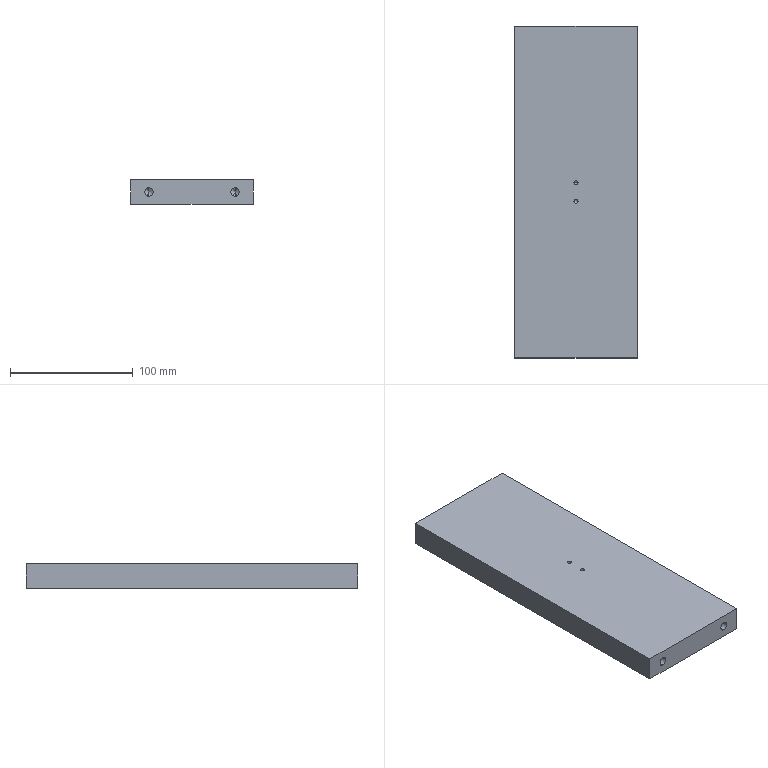Part | SolidWorks | features HoleWzd 3, 3DProfileFeature 1, Extrusion 1 | 1 solid | 42 faces | box 100 x 270 x 20 mm | volume 536586 mm3 | cylinder 18 | cone 18 | plane 6 | commonest cylinder face diameters 3.3 x10 6.8 x8
STEP:
#1=CARTESIAN_POINT('',(61.65,-55.,10.1));
#2=VERTEX_POINT('',#1);
#3=CARTESIAN_POINT('',(58.35,-55.,10.1));
#4=VERTEX_POINT('',#3);
#5=CARTESIAN_POINT('',(60.,-55.,10.1));
#6=DIRECTION('',(0.,0.,-1.));
#7=DIRECTION('',(-1.,0.,0.));
#8=AXIS2_PLACEMENT_3D('',#5,#6,#7);
#9=CIRCLE('',#8,1.65);
#10=EDGE_CURVE('',#2,#4,#9,.T.);
#11=ORIENTED_EDGE('',*,*,#10,.F.);
#12=CARTESIAN_POINT('',(61.65,-55.,0.));
#13=VERTEX_POINT('',#12);
#14=CARTESIAN_POINT('',(61.65,-55.,0.));
#15=DIRECTION('',(0.,0.,-1.));
#16=VECTOR('',#15,1000.);
#17=LINE('',#14,#16);
#18=EDGE_CURVE('',#2,#13,#17,.T.);
#19=ORIENTED_EDGE('',*,*,#18,.T.);
#20=CARTESIAN_POINT('',(58.35,-55.,0.));
#21=VERTEX_POINT('',#20);
#22=CARTESIAN_POINT('',(60.,-55.,0.));
#23=DIRECTION('',(0.,0.,-1.));
#24=DIRECTION('',(-1.,0.,0.));
#25=AXIS2_PLACEMENT_3D('',#22,#23,#24);
#26=CIRCLE('',#25,1.65);
#27=EDGE_CURVE('',#13,#21,#26,.T.);
#28=ORIENTED_EDGE('',*,*,#27,.T.);
#29=CARTESIAN_POINT('',(58.35,-55.,0.));
#30=DIRECTION('',(0.,0.,-1.));
#31=VECTOR('',#30,1000.);
#32=LINE('',#29,#31);
#33=EDGE_CURVE('',#4,#21,#32,.T.);
#34=ORIENTED_EDGE('',*,*,#33,.F.);
#35=EDGE_LOOP('',(#11,#19,#28,#34));
#36=FACE_OUTER_BOUND('',#35,.T.);
#37=CARTESIAN_POINT('',(60.,-55.,0.));
#38=DIRECTION('',(0.,0.,-1.));
#39=DIRECTION('',(-1.,0.,0.));
#40=AXIS2_PLACEMENT_3D('',#37,#38,#39);
#41=CYLINDRICAL_SURFACE('',#40,1.65);
#42=ADVANCED_FACE('',(#36),#41,.F.);
#43=CARTESIAN_POINT('',(60.,-55.,11.091));
#44=VERTEX_POINT('',#43);
#45=CARTESIAN_POINT('',(58.35,-55.,10.1));
#46=DIRECTION('',(-0.8572,0.,-0.515));
#47=VECTOR('',#46,1000.);
#48=LINE('',#45,#47);
#49=EDGE_CURVE('',#44,#4,#48,.T.);
#50=ORIENTED_EDGE('',*,*,#49,.F.);
#51=CARTESIAN_POINT('',(61.65,-55.,10.1));
#52=DIRECTION('',(0.8572,0.,-0.515));
#53=VECTOR('',#52,1000.);
#54=LINE('',#51,#53);
#55=EDGE_CURVE('',#44,#2,#54,.T.);
#56=ORIENTED_EDGE('',*,*,#55,.T.);
#57=ORIENTED_EDGE('',*,*,#10,.T.);
#58=EDGE_LOOP('',(#50,#56,#57));
#59=FACE_OUTER_BOUND('',#58,.T.);
#60=CARTESIAN_POINT('',(60.,-55.,10.1));
#61=DIRECTION('',(0.,0.,-1.));
#62=DIRECTION('',(-1.,0.,0.));
#63=AXIS2_PLACEMENT_3D('',#60,#61,#62);
#64=CONICAL_SURFACE('',#63,1.65,1.03);
#65=ADVANCED_FACE('',(#59),#64,.F.);
#66=CARTESIAN_POINT('',(61.65,-115.,10.1));
#67=VERTEX_POINT('',#66);
#68=CARTESIAN_POINT('',(58.35,-115.,10.1));
#69=VERTEX_POINT('',#68);
#70=CARTESIAN_POINT('',(60.,-115.,10.1));
#71=DIRECTION('',(0.,0.,-1.));
#72=DIRECTION('',(-1.,0.,0.));
#73=AXIS2_PLACEMENT_3D('',#70,#71,#72);
#74=CIRCLE('',#73,1.65);
#75=EDGE_CURVE('',#67,#69,#74,.T.);
#76=ORIENTED_EDGE('',*,*,#75,.F.);
#77=CARTESIAN_POINT('',(61.65,-115.,0.));
#78=VERTEX_POINT('',#77);
#79=CARTESIAN_POINT('',(61.65,-115.,0.));
#80=DIRECTION('',(0.,0.,-1.));
#81=VECTOR('',#80,1000.);
#82=LINE('',#79,#81);
#83=EDGE_CURVE('',#67,#78,#82,.T.);
#84=ORIENTED_EDGE('',*,*,#83,.T.);
#85=CARTESIAN_POINT('',(58.35,-115.,0.));
#86=VERTEX_POINT('',#85);
#87=CARTESIAN_POINT('',(60.,-115.,0.));
#88=DIRECTION('',(0.,0.,-1.));
#89=DIRECTION('',(-1.,0.,0.));
#90=AXIS2_PLACEMENT_3D('',#87,#88,#89);
#91=CIRCLE('',#90,1.65);
#92=EDGE_CURVE('',#78,#86,#91,.T.);
#93=ORIENTED_EDGE('',*,*,#92,.T.);
#94=CARTESIAN_POINT('',(58.35,-115.,0.));
#95=DIRECTION('',(0.,0.,-1.));
#96=VECTOR('',#95,1000.);
#97=LINE('',#94,#96);
#98=EDGE_CURVE('',#69,#86,#97,.T.);
#99=ORIENTED_EDGE('',*,*,#98,.F.);
#100=EDGE_LOOP('',(#76,#84,#93,#99));
#101=FACE_OUTER_BOUND('',#100,.T.);
#102=CARTESIAN_POINT('',(60.,-115.,0.));
#103=DIRECTION('',(0.,0.,-1.));
#104=DIRECTION('',(-1.,0.,0.));
#105=AXIS2_PLACEMENT_3D('',#102,#103,#104);
#106=CYLINDRICAL_SURFACE('',#105,1.65);
#107=ADVANCED_FACE('',(#101),#106,.F.);
#108=CARTESIAN_POINT('',(60.,-115.,11.091));
#109=VERTEX_POINT('',#108);
#110=CARTESIAN_POINT('',(58.35,-115.,10.1));
#111=DIRECTION('',(-0.8572,0.,-0.515));
#112=VECTOR('',#111,1000.);
#113=LINE('',#110,#112);
#114=EDGE_CURVE('',#109,#69,#113,.T.);
#115=ORIENTED_EDGE('',*,*,#114,.F.);
#116=CARTESIAN_POINT('',(61.65,-115.,10.1));
#117=DIRECTION('',(0.8572,0.,-0.515));
#118=VECTOR('',#117,1000.);
#119=LINE('',#116,#118);
#120=EDGE_CURVE('',#109,#67,#119,.T.);
#121=ORIENTED_EDGE('',*,*,#120,.T.);
#122=ORIENTED_EDGE('',*,*,#75,.T.);
#123=EDGE_LOOP('',(#115,#121,#122));
#124=FACE_OUTER_BOUND('',#123,.T.);
#125=CARTESIAN_POINT('',(60.,-115.,10.1));
#126=DIRECTION('',(0.,0.,-1.));
#127=DIRECTION('',(-1.,0.,0.));
#128=AXIS2_PLACEMENT_3D('',#125,#126,#127);
#129=CONICAL_SURFACE('',#128,1.65,1.03);
#130=ADVANCED_FACE('',(#124),#129,.F.);
#131=CARTESIAN_POINT('',(61.65,-175.,10.1));
#132=VERTEX_POINT('',#131);
#133=CARTESIAN_POINT('',(58.35,-175.,10.1));
#134=VERTEX_POINT('',#133);
#135=CARTESIAN_POINT('',(60.,-175.,10.1));
#136=DIRECTION('',(0.,0.,-1.));
#137=DIRECTION('',(-1.,0.,0.));
#138=AXIS2_PLACEMENT_3D('',#135,#136,#137);
#139=CIRCLE('',#138,1.65);
#140=EDGE_CURVE('',#132,#134,#139,.T.);
#141=ORIENTED_EDGE('',*,*,#140,.F.);
#142=CARTESIAN_POINT('',(61.65,-175.,0.));
#143=VERTEX_POINT('',#142);
#144=CARTESIAN_POINT('',(61.65,-175.,0.));
#145=DIRECTION('',(0.,0.,-1.));
#146=VECTOR('',#145,1000.);
#147=LINE('',#144,#146);
#148=EDGE_CURVE('',#132,#143,#147,.T.);
#149=ORIENTED_EDGE('',*,*,#148,.T.);
#150=CARTESIAN_POINT('',(58.35,-175.,0.));
#151=VERTEX_POINT('',#150);
#152=CARTESIAN_POINT('',(60.,-175.,0.));
#153=DIRECTION('',(0.,0.,-1.));
#154=DIRECTION('',(-1.,0.,0.));
#155=AXIS2_PLACEMENT_3D('',#152,#153,#154);
#156=CIRCLE('',#155,1.65);
#157=EDGE_CURVE('',#143,#151,#156,.T.);
#158=ORIENTED_EDGE('',*,*,#157,.T.);
#159=CARTESIAN_POINT('',(58.35,-175.,0.));
#160=DIRECTION('',(0.,0.,-1.));
#161=VECTOR('',#160,1000.);
#162=LINE('',#159,#161);
#163=EDGE_CURVE('',#134,#151,#162,.T.);
#164=ORIENTED_EDGE('',*,*,#163,.F.);
#165=EDGE_LOOP('',(#141,#149,#158,#164));
#166=FACE_OUTER_BOUND('',#165,.T.);
#167=CARTESIAN_POINT('',(60.,-175.,0.));
#168=DIRECTION('',(0.,0.,-1.));
#169=DIRECTION('',(-1.,0.,0.));
#170=AXIS2_PLACEMENT_3D('',#167,#168,#169);
#171=CYLINDRICAL_SURFACE('',#170,1.65);
#172=ADVANCED_FACE('',(#166),#171,.F.);
#173=CARTESIAN_POINT('',(60.,-175.,11.091));
#174=VERTEX_POINT('',#173);
#175=CARTESIAN_POINT('',(58.35,-175.,10.1));
#176=DIRECTION('',(-0.8572,0.,-0.515));
#177=VECTOR('',#176,1000.);
#178=LINE('',#175,#177);
#179=EDGE_CURVE('',#174,#134,#178,.T.);
#180=ORIENTED_EDGE('',*,*,#179,.F.);
#181=CARTESIAN_POINT('',(61.65,-175.,10.1));
#182=DIRECTION('',(0.8572,0.,-0.515));
#183=VECTOR('',#182,1000.);
#184=LINE('',#181,#183);
#185=EDGE_CURVE('',#174,#132,#184,.T.);
#186=ORIENTED_EDGE('',*,*,#185,.T.);
#187=ORIENTED_EDGE('',*,*,#140,.T.);
#188=EDGE_LOOP('',(#180,#186,#187));
#189=FACE_OUTER_BOUND('',#188,.T.);
#190=CARTESIAN_POINT('',(60.,-175.,10.1));
#191=DIRECTION('',(0.,0.,-1.));
#192=DIRECTION('',(-1.,0.,0.));
#193=AXIS2_PLACEMENT_3D('',#190,#191,#192);
#194=CONICAL_SURFACE('',#193,1.65,1.03);
#195=ADVANCED_FACE('',(#189),#194,.F.);
#196=CARTESIAN_POINT('',(48.35,-127.5,9.9));
#197=VERTEX_POINT('',#196);
#198=CARTESIAN_POINT('',(51.65,-127.5,9.9));
#199=VERTEX_POINT('',#198);
#200=CARTESIAN_POINT('',(50.,-127.5,9.9));
#201=DIRECTION('',(0.,0.,1.));
#202=DIRECTION('',(1.,0.,0.));
#203=AXIS2_PLACEMENT_3D('',#200,#201,#202);
#204=CIRCLE('',#203,1.65);
#205=EDGE_CURVE('',#197,#199,#204,.T.);
#206=ORIENTED_EDGE('',*,*,#205,.F.);
#207=CARTESIAN_POINT('',(48.35,-127.5,20.));
#208=VERTEX_POINT('',#207);
#209=CARTESIAN_POINT('',(48.35,-127.5,20.));
#210=DIRECTION('',(0.,0.,1.));
#211=VECTOR('',#210,1000.);
#212=LINE('',#209,#211);
#213=EDGE_CURVE('',#197,#208,#212,.T.);
#214=ORIENTED_EDGE('',*,*,#213,.T.);
#215=CARTESIAN_POINT('',(51.65,-127.5,20.));
#216=VERTEX_POINT('',#215);
#217=CARTESIAN_POINT('',(50.,-127.5,20.));
#218=DIRECTION('',(0.,0.,1.));
#219=DIRECTION('',(1.,0.,0.));
#220=AXIS2_PLACEMENT_3D('',#217,#218,#219);
#221=CIRCLE('',#220,1.65);
#222=EDGE_CURVE('',#208,#216,#221,.T.);
#223=ORIENTED_EDGE('',*,*,#222,.T.);
#224=CARTESIAN_POINT('',(51.65,-127.5,20.));
#225=DIRECTION('',(0.,0.,1.));
#226=VECTOR('',#225,1000.);
#227=LINE('',#224,#226);
#228=EDGE_CURVE('',#199,#216,#227,.T.);
#229=ORIENTED_EDGE('',*,*,#228,.F.);
#230=EDGE_LOOP('',(#206,#214,#223,#229));
#231=FACE_OUTER_BOUND('',#230,.T.);
#232=CARTESIAN_POINT('',(50.,-127.5,20.));
#233=DIRECTION('',(0.,0.,1.));
#234=DIRECTION('',(1.,0.,0.));
#235=AXIS2_PLACEMENT_3D('',#232,#233,#234);
#236=CYLINDRICAL_SURFACE('',#235,1.65);
#237=ADVANCED_FACE('',(#231),#236,.F.);
#238=CARTESIAN_POINT('',(50.,-127.5,8.909));
#239=VERTEX_POINT('',#238);
#240=CARTESIAN_POINT('',(51.65,-127.5,9.9));
#241=DIRECTION('',(0.8572,0.,0.515));
#242=VECTOR('',#241,1000.);
#243=LINE('',#240,#242);
#244=EDGE_CURVE('',#239,#199,#243,.T.);
#245=ORIENTED_EDGE('',*,*,#244,.F.);
#246=CARTESIAN_POINT('',(48.35,-127.5,9.9));
#247=DIRECTION('',(-0.8572,0.,0.515));
#248=VECTOR('',#247,1000.);
#249=LINE('',#246,#248);
#250=EDGE_CURVE('',#239,#197,#249,.T.);
#251=ORIENTED_EDGE('',*,*,#250,.T.);
#252=ORIENTED_EDGE('',*,*,#205,.T.);
#253=EDGE_LOOP('',(#245,#251,#252));
#254=FACE_OUTER_BOUND('',#253,.T.);
#255=CARTESIAN_POINT('',(50.,-127.5,9.9));
#256=DIRECTION('',(0.,0.,1.));
#257=DIRECTION('',(1.,0.,0.));
#258=AXIS2_PLACEMENT_3D('',#255,#256,#257);
#259=CONICAL_SURFACE('',#258,1.65,1.03);
#260=ADVANCED_FACE('',(#254),#259,.F.);
#261=CARTESIAN_POINT('',(48.35,-142.5,9.9));
#262=VERTEX_POINT('',#261);
#263=CARTESIAN_POINT('',(51.65,-142.5,9.9));
#264=VERTEX_POINT('',#263);
#265=CARTESIAN_POINT('',(50.,-142.5,9.9));
#266=DIRECTION('',(0.,0.,1.));
#267=DIRECTION('',(1.,0.,0.));
#268=AXIS2_PLACEMENT_3D('',#265,#266,#267);
#269=CIRCLE('',#268,1.65);
#270=EDGE_CURVE('',#262,#264,#269,.T.);
#271=ORIENTED_EDGE('',*,*,#270,.F.);
#272=CARTESIAN_POINT('',(48.35,-142.5,20.));
#273=VERTEX_POINT('',#272);
#274=CARTESIAN_POINT('',(48.35,-142.5,20.));
#275=DIRECTION('',(0.,0.,1.));
#276=VECTOR('',#275,1000.);
#277=LINE('',#274,#276);
#278=EDGE_CURVE('',#262,#273,#277,.T.);
#279=ORIENTED_EDGE('',*,*,#278,.T.);
#280=CARTESIAN_POINT('',(51.65,-142.5,20.));
#281=VERTEX_POINT('',#280);
#282=CARTESIAN_POINT('',(50.,-142.5,20.));
#283=DIRECTION('',(0.,0.,1.));
#284=DIRECTION('',(1.,0.,0.));
#285=AXIS2_PLACEMENT_3D('',#282,#283,#284);
#286=CIRCLE('',#285,1.65);
#287=EDGE_CURVE('',#273,#281,#286,.T.);
#288=ORIENTED_EDGE('',*,*,#287,.T.);
#289=CARTESIAN_POINT('',(51.65,-142.5,20.));
#290=DIRECTION('',(0.,0.,1.));
#291=VECTOR('',#290,1000.);
#292=LINE('',#289,#291);
#293=EDGE_CURVE('',#264,#281,#292,.T.);
#294=ORIENTED_EDGE('',*,*,#293,.F.);
#295=EDGE_LOOP('',(#271,#279,#288,#294));
#296=FACE_OUTER_BOUND('',#295,.T.);
#297=CARTESIAN_POINT('',(50.,-142.5,20.));
#298=DIRECTION('',(0.,0.,1.));
#299=DIRECTION('',(1.,0.,0.));
#300=AXIS2_PLACEMENT_3D('',#297,#298,#299);
#301=CYLINDRICAL_SURFACE('',#300,1.65);
#302=ADVANCED_FACE('',(#296),#301,.F.);
#303=CARTESIAN_POINT('',(50.,-142.5,8.909));
#304=VERTEX_POINT('',#303);
#305=CARTESIAN_POINT('',(51.65,-142.5,9.9));
#306=DIRECTION('',(0.8572,0.,0.515));
#307=VECTOR('',#306,1000.);
#308=LINE('',#305,#307);
#309=EDGE_CURVE('',#304,#264,#308,.T.);
#310=ORIENTED_EDGE('',*,*,#309,.F.);
#311=CARTESIAN_POINT('',(48.35,-142.5,9.9));
#312=DIRECTION('',(-0.8572,0.,0.515));
#313=VECTOR('',#312,1000.);
#314=LINE('',#311,#313);
#315=EDGE_CURVE('',#304,#262,#314,.T.);
#316=ORIENTED_EDGE('',*,*,#315,.T.);
#317=ORIENTED_EDGE('',*,*,#270,.T.);
#318=EDGE_LOOP('',(#310,#316,#317));
#319=FACE_OUTER_BOUND('',#318,.T.);
#320=CARTESIAN_POINT('',(50.,-142.5,9.9));
#321=DIRECTION('',(0.,0.,1.));
#322=DIRECTION('',(1.,0.,0.));
#323=AXIS2_PLACEMENT_3D('',#320,#321,#322);
#324=CONICAL_SURFACE('',#323,1.65,1.03);
#325=ADVANCED_FACE('',(#319),#324,.F.);
#326=CARTESIAN_POINT('',(15.,-19.75,6.6));
#327=VERTEX_POINT('',#326);
#328=CARTESIAN_POINT('',(15.,-19.75,13.4));
#329=VERTEX_POINT('',#328);
#330=CARTESIAN_POINT('',(15.,-19.75,10.));
#331=DIRECTION('',(0.,1.,0.));
#332=DIRECTION('',(0.,0.,1.));
#333=AXIS2_PLACEMENT_3D('',#330,#331,#332);
#334=CIRCLE('',#333,3.4);
#335=EDGE_CURVE('',#327,#329,#334,.T.);
#336=ORIENTED_EDGE('',*,*,#335,.F.);
#337=CARTESIAN_POINT('',(15.,0.,6.6));
#338=VERTEX_POINT('',#337);
#339=CARTESIAN_POINT('',(15.,0.,6.6));
#340=DIRECTION('',(0.,1.,0.));
#341=VECTOR('',#340,1000.);
#342=LINE('',#339,#341);
#343=EDGE_CURVE('',#327,#338,#342,.T.);
#344=ORIENTED_EDGE('',*,*,#343,.T.);
#345=CARTESIAN_POINT('',(15.,0.,13.4));
#346=VERTEX_POINT('',#345);
#347=CARTESIAN_POINT('',(15.,0.,10.));
#348=DIRECTION('',(0.,1.,0.));
#349=DIRECTION('',(0.,0.,1.));
#350=AXIS2_PLACEMENT_3D('',#347,#348,#349);
#351=CIRCLE('',#350,3.4);
#352=EDGE_CURVE('',#338,#346,#351,.T.);
#353=ORIENTED_EDGE('',*,*,#352,.T.);
#354=CARTESIAN_POINT('',(15.,0.,13.4));
#355=DIRECTION('',(0.,1.,0.));
#356=VECTOR('',#355,1000.);
#357=LINE('',#354,#356);
#358=EDGE_CURVE('',#329,#346,#357,.T.);
#359=ORIENTED_EDGE('',*,*,#358,.F.);
#360=EDGE_LOOP('',(#336,#344,#353,#359));
#361=FACE_OUTER_BOUND('',#360,.T.);
#362=CARTESIAN_POINT('',(15.,0.,10.));
#363=DIRECTION('',(0.,1.,0.));
#364=DIRECTION('',(0.,0.,1.));
#365=AXIS2_PLACEMENT_3D('',#362,#363,#364);
#366=CYLINDRICAL_SURFACE('',#365,3.4);
#367=ADVANCED_FACE('',(#361),#366,.F.);
#368=CARTESIAN_POINT('',(15.,-21.793,10.));
#369=VERTEX_POINT('',#368);
#370=CARTESIAN_POINT('',(15.,-19.75,13.4));
#371=DIRECTION('',(0.,0.515,0.8572));
#372=VECTOR('',#371,1000.);
#373=LINE('',#370,#372);
#374=EDGE_CURVE('',#369,#329,#373,.T.);
#375=ORIENTED_EDGE('',*,*,#374,.F.);
#376=CARTESIAN_POINT('',(15.,-19.75,6.6));
#377=DIRECTION('',(0.,0.515,-0.8572));
#378=VECTOR('',#377,1000.);
#379=LINE('',#376,#378);
#380=EDGE_CURVE('',#369,#327,#379,.T.);
#381=ORIENTED_EDGE('',*,*,#380,.T.);
#382=ORIENTED_EDGE('',*,*,#335,.T.);
#383=EDGE_LOOP('',(#375,#381,#382));
#384=FACE_OUTER_BOUND('',#383,.T.);
#385=CARTESIAN_POINT('',(15.,-19.75,10.));
#386=DIRECTION('',(0.,1.,0.));
#387=DIRECTION('',(0.,0.,1.));
#388=AXIS2_PLACEMENT_3D('',#385,#386,#387);
#389=CONICAL_SURFACE('',#388,3.4,1.03);
#390=ADVANCED_FACE('',(#384),#389,.F.);
#391=CARTESIAN_POINT('',(85.,-19.75,6.6));
#392=VERTEX_POINT('',#391);
#393=CARTESIAN_POINT('',(85.,-19.75,13.4));
#394=VERTEX_POINT('',#393);
#395=CARTESIAN_POINT('',(85.,-19.75,10.));
#396=DIRECTION('',(0.,1.,0.));
#397=DIRECTION('',(0.,0.,1.));
#398=AXIS2_PLACEMENT_3D('',#395,#396,#397);
#399=CIRCLE('',#398,3.4);
#400=EDGE_CURVE('',#392,#394,#399,.T.);
#401=ORIENTED_EDGE('',*,*,#400,.F.);
#402=CARTESIAN_POINT('',(85.,0.,6.6));
#403=VERTEX_POINT('',#402);
#404=CARTESIAN_POINT('',(85.,0.,6.6));
#405=DIRECTION('',(0.,1.,0.));
#406=VECTOR('',#405,1000.);
#407=LINE('',#404,#406);
#408=EDGE_CURVE('',#392,#403,#407,.T.);
#409=ORIENTED_EDGE('',*,*,#408,.T.);
#410=CARTESIAN_POINT('',(85.,0.,13.4));
#411=VERTEX_POINT('',#410);
#412=CARTESIAN_POINT('',(85.,0.,10.));
#413=DIRECTION('',(0.,1.,0.));
#414=DIRECTION('',(0.,0.,1.));
#415=AXIS2_PLACEMENT_3D('',#412,#413,#414);
#416=CIRCLE('',#415,3.4);
#417=EDGE_CURVE('',#403,#411,#416,.T.);
#418=ORIENTED_EDGE('',*,*,#417,.T.);
#419=CARTESIAN_POINT('',(85.,0.,13.4));
#420=DIRECTION('',(0.,1.,0.));
#421=VECTOR('',#420,1000.);
#422=LINE('',#419,#421);
#423=EDGE_CURVE('',#394,#411,#422,.T.);
#424=ORIENTED_EDGE('',*,*,#423,.F.);
#425=EDGE_LOOP('',(#401,#409,#418,#424));
#426=FACE_OUTER_BOUND('',#425,.T.);
#427=CARTESIAN_POINT('',(85.,0.,10.));
#428=DIRECTION('',(0.,1.,0.));
#429=DIRECTION('',(0.,0.,1.));
#430=AXIS2_PLACEMENT_3D('',#427,#428,#429);
#431=CYLINDRICAL_SURFACE('',#430,3.4);
#432=ADVANCED_FACE('',(#426),#431,.F.);
#433=CARTESIAN_POINT('',(85.,-21.793,10.));
#434=VERTEX_POINT('',#433);
#435=CARTESIAN_POINT('',(85.,-19.75,13.4));
#436=DIRECTION('',(0.,0.515,0.8572));
#437=VECTOR('',#436,1000.);
#438=LINE('',#435,#437);
#439=EDGE_CURVE('',#434,#394,#438,.T.);
#440=ORIENTED_EDGE('',*,*,#439,.F.);
#441=CARTESIAN_POINT('',(85.,-19.75,6.6));
#442=DIRECTION('',(0.,0.515,-0.8572));
#443=VECTOR('',#442,1000.);
#444=LINE('',#441,#443);
#445=EDGE_CURVE('',#434,#392,#444,.T.);
#446=ORIENTED_EDGE('',*,*,#445,.T.);
#447=ORIENTED_EDGE('',*,*,#400,.T.);
#448=EDGE_LOOP('',(#440,#446,#447));
#449=FACE_OUTER_BOUND('',#448,.T.);
#450=CARTESIAN_POINT('',(85.,-19.75,10.));
#451=DIRECTION('',(0.,1.,0.));
#452=DIRECTION('',(0.,0.,1.));
#453=AXIS2_PLACEMENT_3D('',#450,#451,#452);
#454=CONICAL_SURFACE('',#453,3.4,1.03);
#455=ADVANCED_FACE('',(#449),#454,.F.);
#456=CARTESIAN_POINT('',(15.,-250.25,13.4));
#457=VERTEX_POINT('',#456);
#458=CARTESIAN_POINT('',(15.,-250.25,6.6));
#459=VERTEX_POINT('',#458);
#460=CARTESIAN_POINT('',(15.,-250.25,10.));
#461=DIRECTION('',(0.,-1.,0.));
#462=DIRECTION('',(0.,0.,-1.));
#463=AXIS2_PLACEMENT_3D('',#460,#461,#462);
#464=CIRCLE('',#463,3.4);
#465=EDGE_CURVE('',#457,#459,#464,.T.);
#466=ORIENTED_EDGE('',*,*,#465,.F.);
#467=CARTESIAN_POINT('',(15.,-270.,13.4));
#468=VERTEX_POINT('',#467);
#469=CARTESIAN_POINT('',(15.,-270.,13.4));
#470=DIRECTION('',(0.,-1.,0.));
#471=VECTOR('',#470,1000.);
#472=LINE('',#469,#471);
#473=EDGE_CURVE('',#457,#468,#472,.T.);
#474=ORIENTED_EDGE('',*,*,#473,.T.);
#475=CARTESIAN_POINT('',(15.,-270.,6.6));
#476=VERTEX_POINT('',#475);
#477=CARTESIAN_POINT('',(15.,-270.,10.));
#478=DIRECTION('',(0.,-1.,0.));
#479=DIRECTION('',(0.,0.,-1.));
#480=AXIS2_PLACEMENT_3D('',#477,#478,#479);
#481=CIRCLE('',#480,3.4);
#482=EDGE_CURVE('',#468,#476,#481,.T.);
#483=ORIENTED_EDGE('',*,*,#482,.T.);
#484=CARTESIAN_POINT('',(15.,-270.,6.6));
#485=DIRECTION('',(0.,-1.,0.));
#486=VECTOR('',#485,1000.);
#487=LINE('',#484,#486);
#488=EDGE_CURVE('',#459,#476,#487,.T.);
#489=ORIENTED_EDGE('',*,*,#488,.F.);
#490=EDGE_LOOP('',(#466,#474,#483,#489));
#491=FACE_OUTER_BOUND('',#490,.T.);
#492=CARTESIAN_POINT('',(15.,-270.,10.));
#493=DIRECTION('',(0.,-1.,0.));
#494=DIRECTION('',(0.,0.,-1.));
#495=AXIS2_PLACEMENT_3D('',#492,#493,#494);
#496=CYLINDRICAL_SURFACE('',#495,3.4);
#497=ADVANCED_FACE('',(#491),#496,.F.);
#498=CARTESIAN_POINT('',(15.,-248.207,10.));
#499=VERTEX_POINT('',#498);
#500=CARTESIAN_POINT('',(15.,-250.25,6.6));
#501=DIRECTION('',(0.,-0.515,-0.8572));
#502=VECTOR('',#501,1000.);
#503=LINE('',#500,#502);
#504=EDGE_CURVE('',#499,#459,#503,.T.);
#505=ORIENTED_EDGE('',*,*,#504,.F.);
#506=CARTESIAN_POINT('',(15.,-250.25,13.4));
#507=DIRECTION('',(0.,-0.515,0.8572));
#508=VECTOR('',#507,1000.);
#509=LINE('',#506,#508);
#510=EDGE_CURVE('',#499,#457,#509,.T.);
#511=ORIENTED_EDGE('',*,*,#510,.T.);
#512=ORIENTED_EDGE('',*,*,#465,.T.);
#513=EDGE_LOOP('',(#505,#511,#512));
#514=FACE_OUTER_BOUND('',#513,.T.);
#515=CARTESIAN_POINT('',(15.,-250.25,10.));
#516=DIRECTION('',(0.,-1.,0.));
#517=DIRECTION('',(0.,0.,-1.));
#518=AXIS2_PLACEMENT_3D('',#515,#516,#517);
#519=CONICAL_SURFACE('',#518,3.4,1.03);
#520=ADVANCED_FACE('',(#514),#519,.F.);
#521=CARTESIAN_POINT('',(85.,-250.25,13.4));
#522=VERTEX_POINT('',#521);
#523=CARTESIAN_POINT('',(85.,-250.25,6.6));
#524=VERTEX_POINT('',#523);
#525=CARTESIAN_POINT('',(85.,-250.25,10.));
#526=DIRECTION('',(0.,-1.,0.));
#527=DIRECTION('',(0.,0.,-1.));
#528=AXIS2_PLACEMENT_3D('',#525,#526,#527);
#529=CIRCLE('',#528,3.4);
#530=EDGE_CURVE('',#522,#524,#529,.T.);
#531=ORIENTED_EDGE('',*,*,#530,.F.);
#532=CARTESIAN_POINT('',(85.,-270.,13.4));
#533=VERTEX_POINT('',#532);
#534=CARTESIAN_POINT('',(85.,-270.,13.4));
#535=DIRECTION('',(0.,-1.,0.));
#536=VECTOR('',#535,1000.);
#537=LINE('',#534,#536);
#538=EDGE_CURVE('',#522,#533,#537,.T.);
#539=ORIENTED_EDGE('',*,*,#538,.T.);
#540=CARTESIAN_POINT('',(85.,-270.,6.6));
#541=VERTEX_POINT('',#540);
#542=CARTESIAN_POINT('',(85.,-270.,10.));
#543=DIRECTION('',(0.,-1.,0.));
#544=DIRECTION('',(0.,0.,-1.));
#545=AXIS2_PLACEMENT_3D('',#542,#543,#544);
#546=CIRCLE('',#545,3.4);
#547=EDGE_CURVE('',#533,#541,#546,.T.);
#548=ORIENTED_EDGE('',*,*,#547,.T.);
#549=CARTESIAN_POINT('',(85.,-270.,6.6));
#550=DIRECTION('',(0.,-1.,0.));
#551=VECTOR('',#550,1000.);
#552=LINE('',#549,#551);
#553=EDGE_CURVE('',#524,#541,#552,.T.);
#554=ORIENTED_EDGE('',*,*,#553,.F.);
#555=EDGE_LOOP('',(#531,#539,#548,#554));
#556=FACE_OUTER_BOUND('',#555,.T.);
#557=CARTESIAN_POINT('',(85.,-270.,10.));
#558=DIRECTION('',(0.,-1.,0.));
#559=DIRECTION('',(0.,0.,-1.));
#560=AXIS2_PLACEMENT_3D('',#557,#558,#559);
#561=CYLINDRICAL_SURFACE('',#560,3.4);
#562=ADVANCED_FACE('',(#556),#561,.F.);
#563=CARTESIAN_POINT('',(85.,-248.207,10.));
#564=VERTEX_POINT('',#563);
#565=CARTESIAN_POINT('',(85.,-250.25,6.6));
#566=DIRECTION('',(0.,-0.515,-0.8572));
#567=VECTOR('',#566,1000.);
#568=LINE('',#565,#567);
#569=EDGE_CURVE('',#564,#524,#568,.T.);
#570=ORIENTED_EDGE('',*,*,#569,.F.);
#571=CARTESIAN_POINT('',(85.,-250.25,13.4));
#572=DIRECTION('',(0.,-0.515,0.8572));
#573=VECTOR('',#572,1000.);
#574=LINE('',#571,#573);
#575=EDGE_CURVE('',#564,#522,#574,.T.);
#576=ORIENTED_EDGE('',*,*,#575,.T.);
#577=ORIENTED_EDGE('',*,*,#530,.T.);
#578=EDGE_LOOP('',(#570,#576,#577));
#579=FACE_OUTER_BOUND('',#578,.T.);
#580=CARTESIAN_POINT('',(85.,-250.25,10.));
#581=DIRECTION('',(0.,-1.,0.));
#582=DIRECTION('',(0.,0.,-1.));
#583=AXIS2_PLACEMENT_3D('',#580,#581,#582);
#584=CONICAL_SURFACE('',#583,3.4,1.03);
#585=ADVANCED_FACE('',(#579),#584,.F.);
#586=CARTESIAN_POINT('',(0.,0.,0.));
#587=VERTEX_POINT('',#586);
#588=CARTESIAN_POINT('',(0.,-270.,0.));
#589=VERTEX_POINT('',#588);
#590=CARTESIAN_POINT('',(0.,0.,0.));
#591=DIRECTION('',(0.,-1.,0.));
#592=VECTOR('',#591,1000.);
#593=LINE('',#590,#592);
#594=EDGE_CURVE('',#587,#589,#593,.T.);
#595=ORIENTED_EDGE('',*,*,#594,.T.);
#596=CARTESIAN_POINT('',(0.,-270.,20.));
#597=VERTEX_POINT('',#596);
#598=CARTESIAN_POINT('',(0.,-270.,20.));
#599=DIRECTION('',(0.,0.,-1.));
#600=VECTOR('',#599,1000.);
#601=LINE('',#598,#600);
#602=EDGE_CURVE('',#597,#589,#601,.T.);
#603=ORIENTED_EDGE('',*,*,#602,.F.);
#604=CARTESIAN_POINT('',(0.,0.,20.));
#605=VERTEX_POINT('',#604);
#606=CARTESIAN_POINT('',(0.,0.,20.));
#607=DIRECTION('',(0.,-1.,0.));
#608=VECTOR('',#607,1000.);
#609=LINE('',#606,#608);
#610=EDGE_CURVE('',#605,#597,#609,.T.);
#611=ORIENTED_EDGE('',*,*,#610,.F.);
#612=CARTESIAN_POINT('',(0.,0.,20.));
#613=DIRECTION('',(0.,0.,-1.));
#614=VECTOR('',#613,1000.);
#615=LINE('',#612,#614);
#616=EDGE_CURVE('',#605,#587,#615,.T.);
#617=ORIENTED_EDGE('',*,*,#616,.T.);
#618=EDGE_LOOP('',(#595,#603,#611,#617));
#619=FACE_OUTER_BOUND('',#618,.T.);
#620=CARTESIAN_POINT('',(0.,0.,20.));
#621=DIRECTION('',(1.,0.,0.));
#622=DIRECTION('',(0.,1.,0.));
#623=AXIS2_PLACEMENT_3D('',#620,#621,#622);
#624=PLANE('',#623);
#625=ADVANCED_FACE('',(#619),#624,.F.);
#626=CARTESIAN_POINT('',(15.,-270.,10.));
#627=DIRECTION('',(0.,-1.,0.));
#628=DIRECTION('',(0.,0.,-1.));
#629=AXIS2_PLACEMENT_3D('',#626,#627,#628);
#630=CIRCLE('',#629,3.4);
#631=EDGE_CURVE('',#476,#468,#630,.T.);
#632=ORIENTED_EDGE('',*,*,#631,.F.);
#633=ORIENTED_EDGE('',*,*,#482,.F.);
#634=EDGE_LOOP('',(#632,#633));
#635=FACE_BOUND('',#634,.T.);
#636=CARTESIAN_POINT('',(85.,-270.,10.));
#637=DIRECTION('',(0.,-1.,0.));
#638=DIRECTION('',(0.,0.,-1.));
#639=AXIS2_PLACEMENT_3D('',#636,#637,#638);
#640=CIRCLE('',#639,3.4);
#641=EDGE_CURVE('',#541,#533,#640,.T.);
#642=ORIENTED_EDGE('',*,*,#641,.F.);
#643=ORIENTED_EDGE('',*,*,#547,.F.);
#644=EDGE_LOOP('',(#642,#643));
#645=FACE_BOUND('',#644,.T.);
#646=CARTESIAN_POINT('',(100.,-270.,0.));
#647=VERTEX_POINT('',#646);
#648=CARTESIAN_POINT('',(0.,-270.,0.));
#649=DIRECTION('',(1.,0.,0.));
#650=VECTOR('',#649,1000.);
#651=LINE('',#648,#650);
#652=EDGE_CURVE('',#589,#647,#651,.T.);
#653=ORIENTED_EDGE('',*,*,#652,.T.);
#654=CARTESIAN_POINT('',(100.,-270.,20.));
#655=VERTEX_POINT('',#654);
#656=CARTESIAN_POINT('',(100.,-270.,20.));
#657=DIRECTION('',(0.,0.,-1.));
#658=VECTOR('',#657,1000.);
#659=LINE('',#656,#658);
#660=EDGE_CURVE('',#655,#647,#659,.T.);
#661=ORIENTED_EDGE('',*,*,#660,.F.);
#662=CARTESIAN_POINT('',(0.,-270.,20.));
#663=DIRECTION('',(1.,0.,0.));
#664=VECTOR('',#663,1000.);
#665=LINE('',#662,#664);
#666=EDGE_CURVE('',#597,#655,#665,.T.);
#667=ORIENTED_EDGE('',*,*,#666,.F.);
#668=ORIENTED_EDGE('',*,*,#602,.T.);
#669=EDGE_LOOP('',(#653,#661,#667,#668));
#670=FACE_OUTER_BOUND('',#669,.T.);
#671=CARTESIAN_POINT('',(0.,-270.,20.));
#672=DIRECTION('',(0.,1.,0.));
#673=DIRECTION('',(0.,0.,1.));
#674=AXIS2_PLACEMENT_3D('',#671,#672,#673);
#675=PLANE('',#674);
#676=ADVANCED_FACE('',(#635,#645,#670),#675,.F.);
#677=CARTESIAN_POINT('',(100.,0.,0.));
#678=VERTEX_POINT('',#677);
#679=CARTESIAN_POINT('',(100.,0.,0.));
#680=DIRECTION('',(0.,1.,0.));
#681=VECTOR('',#680,1000.);
#682=LINE('',#679,#681);
#683=EDGE_CURVE('',#647,#678,#682,.T.);
#684=ORIENTED_EDGE('',*,*,#683,.T.);
#685=CARTESIAN_POINT('',(100.,0.,20.));
#686=VERTEX_POINT('',#685);
#687=CARTESIAN_POINT('',(100.,0.,20.));
#688=DIRECTION('',(0.,0.,-1.));
#689=VECTOR('',#688,1000.);
#690=LINE('',#687,#689);
#691=EDGE_CURVE('',#686,#678,#690,.T.);
#692=ORIENTED_EDGE('',*,*,#691,.F.);
#693=CARTESIAN_POINT('',(100.,0.,20.));
#694=DIRECTION('',(0.,1.,0.));
#695=VECTOR('',#694,1000.);
#696=LINE('',#693,#695);
#697=EDGE_CURVE('',#655,#686,#696,.T.);
#698=ORIENTED_EDGE('',*,*,#697,.F.);
#699=ORIENTED_EDGE('',*,*,#660,.T.);
#700=EDGE_LOOP('',(#684,#692,#698,#699));
#701=FACE_OUTER_BOUND('',#700,.T.);
#702=CARTESIAN_POINT('',(100.,0.,20.));
#703=DIRECTION('',(-1.,0.,0.));
#704=DIRECTION('',(0.,-1.,0.));
#705=AXIS2_PLACEMENT_3D('',#702,#703,#704);
#706=PLANE('',#705);
#707=ADVANCED_FACE('',(#701),#706,.F.);
#708=CARTESIAN_POINT('',(15.,0.,10.));
#709=DIRECTION('',(0.,1.,0.));
#710=DIRECTION('',(0.,0.,1.));
#711=AXIS2_PLACEMENT_3D('',#708,#709,#710);
#712=CIRCLE('',#711,3.4);
#713=EDGE_CURVE('',#346,#338,#712,.T.);
#714=ORIENTED_EDGE('',*,*,#713,.F.);
#715=ORIENTED_EDGE('',*,*,#352,.F.);
#716=EDGE_LOOP('',(#714,#715));
#717=FACE_BOUND('',#716,.T.);
#718=CARTESIAN_POINT('',(85.,0.,10.));
#719=DIRECTION('',(0.,1.,0.));
#720=DIRECTION('',(0.,0.,1.));
#721=AXIS2_PLACEMENT_3D('',#718,#719,#720);
#722=CIRCLE('',#721,3.4);
#723=EDGE_CURVE('',#411,#403,#722,.T.);
#724=ORIENTED_EDGE('',*,*,#723,.F.);
#725=ORIENTED_EDGE('',*,*,#417,.F.);
#726=EDGE_LOOP('',(#724,#725));
#727=FACE_BOUND('',#726,.T.);
#728=CARTESIAN_POINT('',(0.,0.,0.));
#729=DIRECTION('',(-1.,0.,0.));
#730=VECTOR('',#729,1000.);
#731=LINE('',#728,#730);
#732=EDGE_CURVE('',#678,#587,#731,.T.);
#733=ORIENTED_EDGE('',*,*,#732,.T.);
#734=ORIENTED_EDGE('',*,*,#616,.F.);
#735=CARTESIAN_POINT('',(0.,0.,20.));
#736=DIRECTION('',(-1.,0.,0.));
#737=VECTOR('',#736,1000.);
#738=LINE('',#735,#737);
#739=EDGE_CURVE('',#686,#605,#738,.T.);
#740=ORIENTED_EDGE('',*,*,#739,.F.);
#741=ORIENTED_EDGE('',*,*,#691,.T.);
#742=EDGE_LOOP('',(#733,#734,#740,#741));
#743=FACE_OUTER_BOUND('',#742,.T.);
#744=CARTESIAN_POINT('',(0.,0.,20.));
#745=DIRECTION('',(0.,-1.,0.));
#746=DIRECTION('',(0.,0.,-1.));
#747=AXIS2_PLACEMENT_3D('',#744,#745,#746);
#748=PLANE('',#747);
#749=ADVANCED_FACE('',(#717,#727,#743),#748,.F.);
#750=CARTESIAN_POINT('',(50.,-127.5,20.));
#751=DIRECTION('',(0.,0.,1.));
#752=DIRECTION('',(1.,0.,0.));
#753=AXIS2_PLACEMENT_3D('',#750,#751,#752);
#754=CIRCLE('',#753,1.65);
#755=EDGE_CURVE('',#216,#208,#754,.T.);
#756=ORIENTED_EDGE('',*,*,#755,.F.);
#757=ORIENTED_EDGE('',*,*,#222,.F.);
#758=EDGE_LOOP('',(#756,#757));
#759=FACE_BOUND('',#758,.T.);
#760=CARTESIAN_POINT('',(50.,-142.5,20.));
#761=DIRECTION('',(0.,0.,1.));
#762=DIRECTION('',(1.,0.,0.));
#763=AXIS2_PLACEMENT_3D('',#760,#761,#762);
#764=CIRCLE('',#763,1.65);
#765=EDGE_CURVE('',#281,#273,#764,.T.);
#766=ORIENTED_EDGE('',*,*,#765,.F.);
#767=ORIENTED_EDGE('',*,*,#287,.F.);
#768=EDGE_LOOP('',(#766,#767));
#769=FACE_BOUND('',#768,.T.);
#770=ORIENTED_EDGE('',*,*,#610,.T.);
#771=ORIENTED_EDGE('',*,*,#666,.T.);
#772=ORIENTED_EDGE('',*,*,#697,.T.);
#773=ORIENTED_EDGE('',*,*,#739,.T.);
#774=EDGE_LOOP('',(#770,#771,#772,#773));
#775=FACE_OUTER_BOUND('',#774,.T.);
#776=CARTESIAN_POINT('',(0.,0.,20.));
#777=DIRECTION('',(0.,0.,1.));
#778=DIRECTION('',(1.,0.,0.));
#779=AXIS2_PLACEMENT_3D('',#776,#777,#778);
#780=PLANE('',#779);
#781=ADVANCED_FACE('',(#759,#769,#775),#780,.T.);
#782=CARTESIAN_POINT('',(60.,-55.,0.));
#783=DIRECTION('',(0.,0.,-1.));
#784=DIRECTION('',(-1.,0.,0.));
#785=AXIS2_PLACEMENT_3D('',#782,#783,#784);
#786=CIRCLE('',#785,1.65);
#787=EDGE_CURVE('',#21,#13,#786,.T.);
#788=ORIENTED_EDGE('',*,*,#787,.F.);
#789=ORIENTED_EDGE('',*,*,#27,.F.);
#790=EDGE_LOOP('',(#788,#789));
#791=FACE_BOUND('',#790,.T.);
#792=CARTESIAN_POINT('',(60.,-115.,0.));
#793=DIRECTION('',(0.,0.,-1.));
#794=DIRECTION('',(-1.,0.,0.));
#795=AXIS2_PLACEMENT_3D('',#792,#793,#794);
#796=CIRCLE('',#795,1.65);
#797=EDGE_CURVE('',#86,#78,#796,.T.);
#798=ORIENTED_EDGE('',*,*,#797,.F.);
#799=ORIENTED_EDGE('',*,*,#92,.F.);
#800=EDGE_LOOP('',(#798,#799));
#801=FACE_BOUND('',#800,.T.);
#802=CARTESIAN_POINT('',(60.,-175.,0.));
#803=DIRECTION('',(0.,0.,-1.));
#804=DIRECTION('',(-1.,0.,0.));
#805=AXIS2_PLACEMENT_3D('',#802,#803,#804);
#806=CIRCLE('',#805,1.65);
#807=EDGE_CURVE('',#151,#143,#806,.T.);
#808=ORIENTED_EDGE('',*,*,#807,.F.);
#809=ORIENTED_EDGE('',*,*,#157,.F.);
#810=EDGE_LOOP('',(#808,#809));
#811=FACE_BOUND('',#810,.T.);
#812=ORIENTED_EDGE('',*,*,#594,.F.);
#813=ORIENTED_EDGE('',*,*,#732,.F.);
#814=ORIENTED_EDGE('',*,*,#683,.F.);
#815=ORIENTED_EDGE('',*,*,#652,.F.);
#816=EDGE_LOOP('',(#812,#813,#814,#815));
#817=FACE_OUTER_BOUND('',#816,.T.);
#818=CARTESIAN_POINT('',(0.,0.,0.));
#819=DIRECTION('',(0.,0.,1.));
#820=DIRECTION('',(1.,0.,0.));
#821=AXIS2_PLACEMENT_3D('',#818,#819,#820);
#822=PLANE('',#821);
#823=ADVANCED_FACE('',(#791,#801,#811,#817),#822,.F.);
#824=ORIENTED_EDGE('',*,*,#575,.F.);
#825=ORIENTED_EDGE('',*,*,#569,.T.);
#826=CARTESIAN_POINT('',(85.,-250.25,10.));
#827=DIRECTION('',(0.,-1.,0.));
#828=DIRECTION('',(0.,0.,-1.));
#829=AXIS2_PLACEMENT_3D('',#826,#827,#828);
#830=CIRCLE('',#829,3.4);
#831=EDGE_CURVE('',#524,#522,#830,.T.);
#832=ORIENTED_EDGE('',*,*,#831,.T.);
#833=EDGE_LOOP('',(#824,#825,#832));
#834=FACE_OUTER_BOUND('',#833,.T.);
#835=CARTESIAN_POINT('',(85.,-250.25,10.));
#836=DIRECTION('',(0.,-1.,0.));
#837=DIRECTION('',(0.,0.,-1.));
#838=AXIS2_PLACEMENT_3D('',#835,#836,#837);
#839=CONICAL_SURFACE('',#838,3.4,1.03);
#840=ADVANCED_FACE('',(#834),#839,.F.);
#841=ORIENTED_EDGE('',*,*,#538,.F.);
#842=ORIENTED_EDGE('',*,*,#831,.F.);
#843=ORIENTED_EDGE('',*,*,#553,.T.);
#844=ORIENTED_EDGE('',*,*,#641,.T.);
#845=EDGE_LOOP('',(#841,#842,#843,#844));
#846=FACE_OUTER_BOUND('',#845,.T.);
#847=CARTESIAN_POINT('',(85.,-270.,10.));
#848=DIRECTION('',(0.,-1.,0.));
#849=DIRECTION('',(0.,0.,-1.));
#850=AXIS2_PLACEMENT_3D('',#847,#848,#849);
#851=CYLINDRICAL_SURFACE('',#850,3.4);
#852=ADVANCED_FACE('',(#846),#851,.F.);
#853=ORIENTED_EDGE('',*,*,#510,.F.);
#854=ORIENTED_EDGE('',*,*,#504,.T.);
#855=CARTESIAN_POINT('',(15.,-250.25,10.));
#856=DIRECTION('',(0.,-1.,0.));
#857=DIRECTION('',(0.,0.,-1.));
#858=AXIS2_PLACEMENT_3D('',#855,#856,#857);
#859=CIRCLE('',#858,3.4);
#860=EDGE_CURVE('',#459,#457,#859,.T.);
#861=ORIENTED_EDGE('',*,*,#860,.T.);
#862=EDGE_LOOP('',(#853,#854,#861));
#863=FACE_OUTER_BOUND('',#862,.T.);
#864=CARTESIAN_POINT('',(15.,-250.25,10.));
#865=DIRECTION('',(0.,-1.,0.));
#866=DIRECTION('',(0.,0.,-1.));
#867=AXIS2_PLACEMENT_3D('',#864,#865,#866);
#868=CONICAL_SURFACE('',#867,3.4,1.03);
#869=ADVANCED_FACE('',(#863),#868,.F.);
#870=ORIENTED_EDGE('',*,*,#473,.F.);
#871=ORIENTED_EDGE('',*,*,#860,.F.);
#872=ORIENTED_EDGE('',*,*,#488,.T.);
#873=ORIENTED_EDGE('',*,*,#631,.T.);
#874=EDGE_LOOP('',(#870,#871,#872,#873));
#875=FACE_OUTER_BOUND('',#874,.T.);
#876=CARTESIAN_POINT('',(15.,-270.,10.));
#877=DIRECTION('',(0.,-1.,0.));
#878=DIRECTION('',(0.,0.,-1.));
#879=AXIS2_PLACEMENT_3D('',#876,#877,#878);
#880=CYLINDRICAL_SURFACE('',#879,3.4);
#881=ADVANCED_FACE('',(#875),#880,.F.);
#882=ORIENTED_EDGE('',*,*,#445,.F.);
#883=ORIENTED_EDGE('',*,*,#439,.T.);
#884=CARTESIAN_POINT('',(85.,-19.75,10.));
#885=DIRECTION('',(0.,1.,0.));
#886=DIRECTION('',(0.,0.,1.));
#887=AXIS2_PLACEMENT_3D('',#884,#885,#886);
#888=CIRCLE('',#887,3.4);
#889=EDGE_CURVE('',#394,#392,#888,.T.);
#890=ORIENTED_EDGE('',*,*,#889,.T.);
#891=EDGE_LOOP('',(#882,#883,#890));
#892=FACE_OUTER_BOUND('',#891,.T.);
#893=CARTESIAN_POINT('',(85.,-19.75,10.));
#894=DIRECTION('',(0.,1.,0.));
#895=DIRECTION('',(0.,0.,1.));
#896=AXIS2_PLACEMENT_3D('',#893,#894,#895);
#897=CONICAL_SURFACE('',#896,3.4,1.03);
#898=ADVANCED_FACE('',(#892),#897,.F.);
#899=ORIENTED_EDGE('',*,*,#408,.F.);
#900=ORIENTED_EDGE('',*,*,#889,.F.);
#901=ORIENTED_EDGE('',*,*,#423,.T.);
#902=ORIENTED_EDGE('',*,*,#723,.T.);
#903=EDGE_LOOP('',(#899,#900,#901,#902));
#904=FACE_OUTER_BOUND('',#903,.T.);
#905=CARTESIAN_POINT('',(85.,0.,10.));
#906=DIRECTION('',(0.,1.,0.));
#907=DIRECTION('',(0.,0.,1.));
#908=AXIS2_PLACEMENT_3D('',#905,#906,#907);
#909=CYLINDRICAL_SURFACE('',#908,3.4);
#910=ADVANCED_FACE('',(#904),#909,.F.);
#911=ORIENTED_EDGE('',*,*,#380,.F.);
#912=ORIENTED_EDGE('',*,*,#374,.T.);
#913=CARTESIAN_POINT('',(15.,-19.75,10.));
#914=DIRECTION('',(0.,1.,0.));
#915=DIRECTION('',(0.,0.,1.));
#916=AXIS2_PLACEMENT_3D('',#913,#914,#915);
#917=CIRCLE('',#916,3.4);
#918=EDGE_CURVE('',#329,#327,#917,.T.);
#919=ORIENTED_EDGE('',*,*,#918,.T.);
#920=EDGE_LOOP('',(#911,#912,#919));
#921=FACE_OUTER_BOUND('',#920,.T.);
#922=CARTESIAN_POINT('',(15.,-19.75,10.));
#923=DIRECTION('',(0.,1.,0.));
#924=DIRECTION('',(0.,0.,1.));
#925=AXIS2_PLACEMENT_3D('',#922,#923,#924);
#926=CONICAL_SURFACE('',#925,3.4,1.03);
#927=ADVANCED_FACE('',(#921),#926,.F.);
#928=ORIENTED_EDGE('',*,*,#343,.F.);
#929=ORIENTED_EDGE('',*,*,#918,.F.);
#930=ORIENTED_EDGE('',*,*,#358,.T.);
#931=ORIENTED_EDGE('',*,*,#713,.T.);
#932=EDGE_LOOP('',(#928,#929,#930,#931));
#933=FACE_OUTER_BOUND('',#932,.T.);
#934=CARTESIAN_POINT('',(15.,0.,10.));
#935=DIRECTION('',(0.,1.,0.));
#936=DIRECTION('',(0.,0.,1.));
#937=AXIS2_PLACEMENT_3D('',#934,#935,#936);
#938=CYLINDRICAL_SURFACE('',#937,3.4);
#939=ADVANCED_FACE('',(#933),#938,.F.);
#940=ORIENTED_EDGE('',*,*,#315,.F.);
#941=ORIENTED_EDGE('',*,*,#309,.T.);
#942=CARTESIAN_POINT('',(50.,-142.5,9.9));
#943=DIRECTION('',(0.,0.,1.));
#944=DIRECTION('',(1.,0.,0.));
#945=AXIS2_PLACEMENT_3D('',#942,#943,#944);
#946=CIRCLE('',#945,1.65);
#947=EDGE_CURVE('',#264,#262,#946,.T.);
#948=ORIENTED_EDGE('',*,*,#947,.T.);
#949=EDGE_LOOP('',(#940,#941,#948));
#950=FACE_OUTER_BOUND('',#949,.T.);
#951=CARTESIAN_POINT('',(50.,-142.5,9.9));
#952=DIRECTION('',(0.,0.,1.));
#953=DIRECTION('',(1.,0.,0.));
#954=AXIS2_PLACEMENT_3D('',#951,#952,#953);
#955=CONICAL_SURFACE('',#954,1.65,1.03);
#956=ADVANCED_FACE('',(#950),#955,.F.);
#957=ORIENTED_EDGE('',*,*,#278,.F.);
#958=ORIENTED_EDGE('',*,*,#947,.F.);
#959=ORIENTED_EDGE('',*,*,#293,.T.);
#960=ORIENTED_EDGE('',*,*,#765,.T.);
#961=EDGE_LOOP('',(#957,#958,#959,#960));
#962=FACE_OUTER_BOUND('',#961,.T.);
#963=CARTESIAN_POINT('',(50.,-142.5,20.));
#964=DIRECTION('',(0.,0.,1.));
#965=DIRECTION('',(1.,0.,0.));
#966=AXIS2_PLACEMENT_3D('',#963,#964,#965);
#967=CYLINDRICAL_SURFACE('',#966,1.65);
#968=ADVANCED_FACE('',(#962),#967,.F.);
#969=ORIENTED_EDGE('',*,*,#250,.F.);
#970=ORIENTED_EDGE('',*,*,#244,.T.);
#971=CARTESIAN_POINT('',(50.,-127.5,9.9));
#972=DIRECTION('',(0.,0.,1.));
#973=DIRECTION('',(1.,0.,0.));
#974=AXIS2_PLACEMENT_3D('',#971,#972,#973);
#975=CIRCLE('',#974,1.65);
#976=EDGE_CURVE('',#199,#197,#975,.T.);
#977=ORIENTED_EDGE('',*,*,#976,.T.);
#978=EDGE_LOOP('',(#969,#970,#977));
#979=FACE_OUTER_BOUND('',#978,.T.);
#980=CARTESIAN_POINT('',(50.,-127.5,9.9));
#981=DIRECTION('',(0.,0.,1.));
#982=DIRECTION('',(1.,0.,0.));
#983=AXIS2_PLACEMENT_3D('',#980,#981,#982);
#984=CONICAL_SURFACE('',#983,1.65,1.03);
#985=ADVANCED_FACE('',(#979),#984,.F.);
#986=ORIENTED_EDGE('',*,*,#213,.F.);
#987=ORIENTED_EDGE('',*,*,#976,.F.);
#988=ORIENTED_EDGE('',*,*,#228,.T.);
#989=ORIENTED_EDGE('',*,*,#755,.T.);
#990=EDGE_LOOP('',(#986,#987,#988,#989));
#991=FACE_OUTER_BOUND('',#990,.T.);
#992=CARTESIAN_POINT('',(50.,-127.5,20.));
#993=DIRECTION('',(0.,0.,1.));
#994=DIRECTION('',(1.,0.,0.));
#995=AXIS2_PLACEMENT_3D('',#992,#993,#994);
#996=CYLINDRICAL_SURFACE('',#995,1.65);
#997=ADVANCED_FACE('',(#991),#996,.F.);
#998=ORIENTED_EDGE('',*,*,#185,.F.);
#999=ORIENTED_EDGE('',*,*,#179,.T.);
#1000=CARTESIAN_POINT('',(60.,-175.,10.1));
#1001=DIRECTION('',(0.,0.,-1.));
#1002=DIRECTION('',(-1.,0.,0.));
#1003=AXIS2_PLACEMENT_3D('',#1000,#1001,#1002);
#1004=CIRCLE('',#1003,1.65);
#1005=EDGE_CURVE('',#134,#132,#1004,.T.);
#1006=ORIENTED_EDGE('',*,*,#1005,.T.);
#1007=EDGE_LOOP('',(#998,#999,#1006));
#1008=FACE_OUTER_BOUND('',#1007,.T.);
#1009=CARTESIAN_POINT('',(60.,-175.,10.1));
#1010=DIRECTION('',(0.,0.,-1.));
#1011=DIRECTION('',(-1.,0.,0.));
#1012=AXIS2_PLACEMENT_3D('',#1009,#1010,#1011);
#1013=CONICAL_SURFACE('',#1012,1.65,1.03);
#1014=ADVANCED_FACE('',(#1008),#1013,.F.);
#1015=ORIENTED_EDGE('',*,*,#148,.F.);
#1016=ORIENTED_EDGE('',*,*,#1005,.F.);
#1017=ORIENTED_EDGE('',*,*,#163,.T.);
#1018=ORIENTED_EDGE('',*,*,#807,.T.);
#1019=EDGE_LOOP('',(#1015,#1016,#1017,#1018));
#1020=FACE_OUTER_BOUND('',#1019,.T.);
#1021=CARTESIAN_POINT('',(60.,-175.,0.));
#1022=DIRECTION('',(0.,0.,-1.));
#1023=DIRECTION('',(-1.,0.,0.));
#1024=AXIS2_PLACEMENT_3D('',#1021,#1022,#1023);
#1025=CYLINDRICAL_SURFACE('',#1024,1.65);
#1026=ADVANCED_FACE('',(#1020),#1025,.F.);
#1027=ORIENTED_EDGE('',*,*,#120,.F.);
#1028=ORIENTED_EDGE('',*,*,#114,.T.);
#1029=CARTESIAN_POINT('',(60.,-115.,10.1));
#1030=DIRECTION('',(0.,0.,-1.));
#1031=DIRECTION('',(-1.,0.,0.));
#1032=AXIS2_PLACEMENT_3D('',#1029,#1030,#1031);
#1033=CIRCLE('',#1032,1.65);
#1034=EDGE_CURVE('',#69,#67,#1033,.T.);
#1035=ORIENTED_EDGE('',*,*,#1034,.T.);
#1036=EDGE_LOOP('',(#1027,#1028,#1035));
#1037=FACE_OUTER_BOUND('',#1036,.T.);
#1038=CARTESIAN_POINT('',(60.,-115.,10.1));
#1039=DIRECTION('',(0.,0.,-1.));
#1040=DIRECTION('',(-1.,0.,0.));
#1041=AXIS2_PLACEMENT_3D('',#1038,#1039,#1040);
#1042=CONICAL_SURFACE('',#1041,1.65,1.03);
#1043=ADVANCED_FACE('',(#1037),#1042,.F.);
#1044=ORIENTED_EDGE('',*,*,#83,.F.);
#1045=ORIENTED_EDGE('',*,*,#1034,.F.);
#1046=ORIENTED_EDGE('',*,*,#98,.T.);
#1047=ORIENTED_EDGE('',*,*,#797,.T.);
#1048=EDGE_LOOP('',(#1044,#1045,#1046,#1047));
#1049=FACE_OUTER_BOUND('',#1048,.T.);
#1050=CARTESIAN_POINT('',(60.,-115.,0.));
#1051=DIRECTION('',(0.,0.,-1.));
#1052=DIRECTION('',(-1.,0.,0.));
#1053=AXIS2_PLACEMENT_3D('',#1050,#1051,#1052);
#1054=CYLINDRICAL_SURFACE('',#1053,1.65);
#1055=ADVANCED_FACE('',(#1049),#1054,.F.);
#1056=ORIENTED_EDGE('',*,*,#55,.F.);
#1057=ORIENTED_EDGE('',*,*,#49,.T.);
#1058=CARTESIAN_POINT('',(60.,-55.,10.1));
#1059=DIRECTION('',(0.,0.,-1.));
#1060=DIRECTION('',(-1.,0.,0.));
#1061=AXIS2_PLACEMENT_3D('',#1058,#1059,#1060);
#1062=CIRCLE('',#1061,1.65);
#1063=EDGE_CURVE('',#4,#2,#1062,.T.);
#1064=ORIENTED_EDGE('',*,*,#1063,.T.);
#1065=EDGE_LOOP('',(#1056,#1057,#1064));
#1066=FACE_OUTER_BOUND('',#1065,.T.);
#1067=CARTESIAN_POINT('',(60.,-55.,10.1));
#1068=DIRECTION('',(0.,0.,-1.));
#1069=DIRECTION('',(-1.,0.,0.));
#1070=AXIS2_PLACEMENT_3D('',#1067,#1068,#1069);
#1071=CONICAL_SURFACE('',#1070,1.65,1.03);
#1072=ADVANCED_FACE('',(#1066),#1071,.F.);
#1073=ORIENTED_EDGE('',*,*,#18,.F.);
#1074=ORIENTED_EDGE('',*,*,#1063,.F.);
#1075=ORIENTED_EDGE('',*,*,#33,.T.);
#1076=ORIENTED_EDGE('',*,*,#787,.T.);
#1077=EDGE_LOOP('',(#1073,#1074,#1075,#1076));
#1078=FACE_OUTER_BOUND('',#1077,.T.);
#1079=CARTESIAN_POINT('',(60.,-55.,0.));
#1080=DIRECTION('',(0.,0.,-1.));
#1081=DIRECTION('',(-1.,0.,0.));
#1082=AXIS2_PLACEMENT_3D('',#1079,#1080,#1081);
#1083=CYLINDRICAL_SURFACE('',#1082,1.65);
#1084=ADVANCED_FACE('',(#1078),#1083,.F.);
#1085=CLOSED_SHELL('',(#42,#65,#107,#130,#172,#195,#237,#260,#302,#325,#367,#390,#432,#455,#497,#520,#562,#585,#625,#676,#707,#749,#781,#823,#840,#852,#869,#881,#898,#910,#927,#939,#956,#968,#985,#997,#1014,#1026,#1043,#1055,#1072,#1084));
#1086=MANIFOLD_SOLID_BREP('',#1085);
#1087=CARTESIAN_POINT('',(0.,0.,0.));
#1088=DIRECTION('',(0.,0.,1.));
#1089=DIRECTION('',(1.,0.,0.));
#1090=AXIS2_PLACEMENT_3D('',#1087,#1088,#1089);
#1091=(LENGTH_UNIT()NAMED_UNIT(*)SI_UNIT(.MILLI.,.METRE.));
#1092=UNCERTAINTY_MEASURE_WITH_UNIT(LENGTH_MEASURE(0.00001),#1091,'','');
#1093=(NAMED_UNIT(*)PLANE_ANGLE_UNIT()SI_UNIT($,.RADIAN.));
#1094=(NAMED_UNIT(*)SI_UNIT($,.STERADIAN.)SOLID_ANGLE_UNIT());
#1095=(GEOMETRIC_REPRESENTATION_CONTEXT(3)GLOBAL_UNCERTAINTY_ASSIGNED_CONTEXT((#1092))GLOBAL_UNIT_ASSIGNED_CONTEXT((#1091,#1093,#1094))REPRESENTATION_CONTEXT('',''));
#1096=ADVANCED_BREP_SHAPE_REPRESENTATION('',(#1086,#1090),#1095);